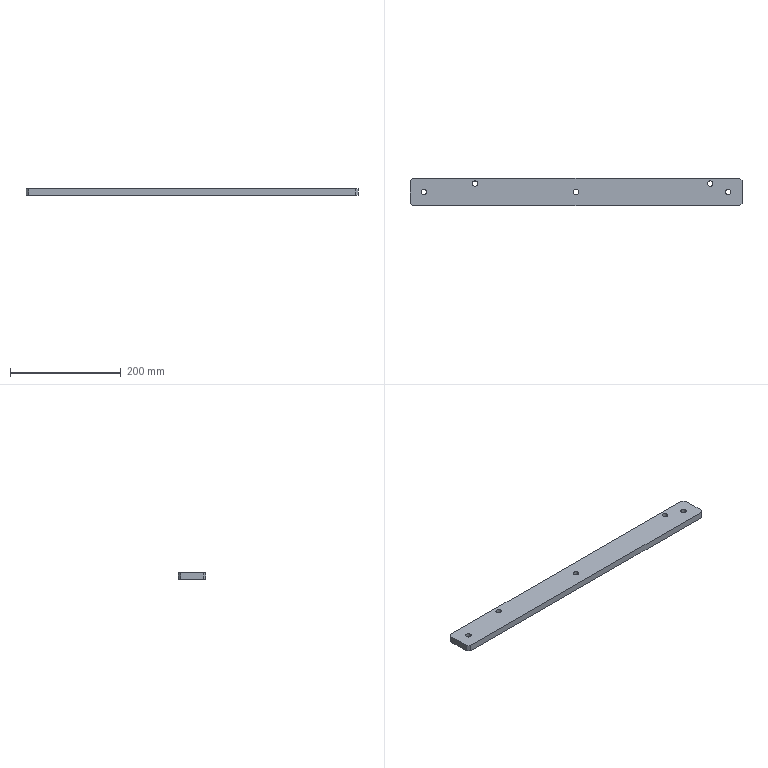Part | STEP file | [01]-6 | 1 solid | 20 faces | box 600 x 50 x 12 mm | volume 354688 mm3 | cylinder 10 | plane 10 | commonest cylinder face diameters 10 x10
STEP:
#1=CARTESIAN_POINT('',(112.5,40.,0.));
#2=VERTEX_POINT('',#1);
#3=CARTESIAN_POINT('',(122.5,40.,0.));
#4=VERTEX_POINT('',#3);
#5=CARTESIAN_POINT('',(117.5,40.,0.));
#6=DIRECTION('',(0.,0.,1.));
#7=DIRECTION('',(1.,0.,0.));
#8=AXIS2_PLACEMENT_3D('',#5,#6,#7);
#9=CIRCLE('',#8,5.);
#10=EDGE_CURVE('',#2,#4,#9,.T.);
#11=ORIENTED_EDGE('',*,*,#10,.F.);
#12=CARTESIAN_POINT('',(112.5,40.,12.));
#13=VERTEX_POINT('',#12);
#14=CARTESIAN_POINT('',(112.5,40.,0.));
#15=DIRECTION('',(0.,0.,1.));
#16=VECTOR('',#15,1000.);
#17=LINE('',#14,#16);
#18=EDGE_CURVE('',#2,#13,#17,.T.);
#19=ORIENTED_EDGE('',*,*,#18,.T.);
#20=CARTESIAN_POINT('',(122.5,40.,12.));
#21=VERTEX_POINT('',#20);
#22=CARTESIAN_POINT('',(117.5,40.,12.));
#23=DIRECTION('',(0.,0.,-1.));
#24=DIRECTION('',(-1.,0.,0.));
#25=AXIS2_PLACEMENT_3D('',#22,#23,#24);
#26=CIRCLE('',#25,5.);
#27=EDGE_CURVE('',#21,#13,#26,.T.);
#28=ORIENTED_EDGE('',*,*,#27,.F.);
#29=CARTESIAN_POINT('',(122.5,40.,0.));
#30=DIRECTION('',(0.,0.,1.));
#31=VECTOR('',#30,1000.);
#32=LINE('',#29,#31);
#33=EDGE_CURVE('',#4,#21,#32,.T.);
#34=ORIENTED_EDGE('',*,*,#33,.F.);
#35=EDGE_LOOP('',(#11,#19,#28,#34));
#36=FACE_OUTER_BOUND('',#35,.T.);
#37=CARTESIAN_POINT('',(117.5,40.,0.));
#38=DIRECTION('',(0.,0.,1.));
#39=DIRECTION('',(1.,0.,0.));
#40=AXIS2_PLACEMENT_3D('',#37,#38,#39);
#41=CYLINDRICAL_SURFACE('',#40,5.);
#42=ADVANCED_FACE('',(#36),#41,.F.);
#43=CARTESIAN_POINT('',(537.5,40.,0.));
#44=VERTEX_POINT('',#43);
#45=CARTESIAN_POINT('',(547.5,40.,0.));
#46=VERTEX_POINT('',#45);
#47=CARTESIAN_POINT('',(542.5,40.,0.));
#48=DIRECTION('',(0.,0.,1.));
#49=DIRECTION('',(1.,0.,0.));
#50=AXIS2_PLACEMENT_3D('',#47,#48,#49);
#51=CIRCLE('',#50,5.);
#52=EDGE_CURVE('',#44,#46,#51,.T.);
#53=ORIENTED_EDGE('',*,*,#52,.F.);
#54=CARTESIAN_POINT('',(537.5,40.,12.));
#55=VERTEX_POINT('',#54);
#56=CARTESIAN_POINT('',(537.5,40.,0.));
#57=DIRECTION('',(0.,0.,1.));
#58=VECTOR('',#57,1000.);
#59=LINE('',#56,#58);
#60=EDGE_CURVE('',#44,#55,#59,.T.);
#61=ORIENTED_EDGE('',*,*,#60,.T.);
#62=CARTESIAN_POINT('',(547.5,40.,12.));
#63=VERTEX_POINT('',#62);
#64=CARTESIAN_POINT('',(542.5,40.,12.));
#65=DIRECTION('',(0.,0.,-1.));
#66=DIRECTION('',(-1.,0.,0.));
#67=AXIS2_PLACEMENT_3D('',#64,#65,#66);
#68=CIRCLE('',#67,5.);
#69=EDGE_CURVE('',#63,#55,#68,.T.);
#70=ORIENTED_EDGE('',*,*,#69,.F.);
#71=CARTESIAN_POINT('',(547.5,40.,0.));
#72=DIRECTION('',(0.,0.,1.));
#73=VECTOR('',#72,1000.);
#74=LINE('',#71,#73);
#75=EDGE_CURVE('',#46,#63,#74,.T.);
#76=ORIENTED_EDGE('',*,*,#75,.F.);
#77=EDGE_LOOP('',(#53,#61,#70,#76));
#78=FACE_OUTER_BOUND('',#77,.T.);
#79=CARTESIAN_POINT('',(542.5,40.,0.));
#80=DIRECTION('',(0.,0.,1.));
#81=DIRECTION('',(1.,0.,0.));
#82=AXIS2_PLACEMENT_3D('',#79,#80,#81);
#83=CYLINDRICAL_SURFACE('',#82,5.);
#84=ADVANCED_FACE('',(#78),#83,.F.);
#85=CARTESIAN_POINT('',(20.,25.,0.));
#86=VERTEX_POINT('',#85);
#87=CARTESIAN_POINT('',(30.,25.,0.));
#88=VERTEX_POINT('',#87);
#89=CARTESIAN_POINT('',(25.,25.,0.));
#90=DIRECTION('',(0.,0.,1.));
#91=DIRECTION('',(1.,0.,0.));
#92=AXIS2_PLACEMENT_3D('',#89,#90,#91);
#93=CIRCLE('',#92,5.);
#94=EDGE_CURVE('',#86,#88,#93,.T.);
#95=ORIENTED_EDGE('',*,*,#94,.F.);
#96=CARTESIAN_POINT('',(20.,25.,12.));
#97=VERTEX_POINT('',#96);
#98=CARTESIAN_POINT('',(20.,25.,0.));
#99=DIRECTION('',(0.,0.,1.));
#100=VECTOR('',#99,1000.);
#101=LINE('',#98,#100);
#102=EDGE_CURVE('',#86,#97,#101,.T.);
#103=ORIENTED_EDGE('',*,*,#102,.T.);
#104=CARTESIAN_POINT('',(30.,25.,12.));
#105=VERTEX_POINT('',#104);
#106=CARTESIAN_POINT('',(25.,25.,12.));
#107=DIRECTION('',(0.,0.,-1.));
#108=DIRECTION('',(-1.,0.,0.));
#109=AXIS2_PLACEMENT_3D('',#106,#107,#108);
#110=CIRCLE('',#109,5.);
#111=EDGE_CURVE('',#105,#97,#110,.T.);
#112=ORIENTED_EDGE('',*,*,#111,.F.);
#113=CARTESIAN_POINT('',(30.,25.,0.));
#114=DIRECTION('',(0.,0.,1.));
#115=VECTOR('',#114,1000.);
#116=LINE('',#113,#115);
#117=EDGE_CURVE('',#88,#105,#116,.T.);
#118=ORIENTED_EDGE('',*,*,#117,.F.);
#119=EDGE_LOOP('',(#95,#103,#112,#118));
#120=FACE_OUTER_BOUND('',#119,.T.);
#121=CARTESIAN_POINT('',(25.,25.,0.));
#122=DIRECTION('',(0.,0.,1.));
#123=DIRECTION('',(1.,0.,0.));
#124=AXIS2_PLACEMENT_3D('',#121,#122,#123);
#125=CYLINDRICAL_SURFACE('',#124,5.);
#126=ADVANCED_FACE('',(#120),#125,.F.);
#127=CARTESIAN_POINT('',(295.,25.,0.));
#128=VERTEX_POINT('',#127);
#129=CARTESIAN_POINT('',(305.,25.,0.));
#130=VERTEX_POINT('',#129);
#131=CARTESIAN_POINT('',(300.,25.,0.));
#132=DIRECTION('',(0.,0.,1.));
#133=DIRECTION('',(1.,0.,0.));
#134=AXIS2_PLACEMENT_3D('',#131,#132,#133);
#135=CIRCLE('',#134,5.);
#136=EDGE_CURVE('',#128,#130,#135,.T.);
#137=ORIENTED_EDGE('',*,*,#136,.F.);
#138=CARTESIAN_POINT('',(295.,25.,12.));
#139=VERTEX_POINT('',#138);
#140=CARTESIAN_POINT('',(295.,25.,0.));
#141=DIRECTION('',(0.,0.,1.));
#142=VECTOR('',#141,1000.);
#143=LINE('',#140,#142);
#144=EDGE_CURVE('',#128,#139,#143,.T.);
#145=ORIENTED_EDGE('',*,*,#144,.T.);
#146=CARTESIAN_POINT('',(305.,25.,12.));
#147=VERTEX_POINT('',#146);
#148=CARTESIAN_POINT('',(300.,25.,12.));
#149=DIRECTION('',(0.,0.,-1.));
#150=DIRECTION('',(-1.,0.,0.));
#151=AXIS2_PLACEMENT_3D('',#148,#149,#150);
#152=CIRCLE('',#151,5.);
#153=EDGE_CURVE('',#147,#139,#152,.T.);
#154=ORIENTED_EDGE('',*,*,#153,.F.);
#155=CARTESIAN_POINT('',(305.,25.,0.));
#156=DIRECTION('',(0.,0.,1.));
#157=VECTOR('',#156,1000.);
#158=LINE('',#155,#157);
#159=EDGE_CURVE('',#130,#147,#158,.T.);
#160=ORIENTED_EDGE('',*,*,#159,.F.);
#161=EDGE_LOOP('',(#137,#145,#154,#160));
#162=FACE_OUTER_BOUND('',#161,.T.);
#163=CARTESIAN_POINT('',(300.,25.,0.));
#164=DIRECTION('',(0.,0.,1.));
#165=DIRECTION('',(1.,0.,0.));
#166=AXIS2_PLACEMENT_3D('',#163,#164,#165);
#167=CYLINDRICAL_SURFACE('',#166,5.);
#168=ADVANCED_FACE('',(#162),#167,.F.);
#169=CARTESIAN_POINT('',(570.,25.,0.));
#170=VERTEX_POINT('',#169);
#171=CARTESIAN_POINT('',(580.,25.,0.));
#172=VERTEX_POINT('',#171);
#173=CARTESIAN_POINT('',(575.,25.,0.));
#174=DIRECTION('',(0.,0.,1.));
#175=DIRECTION('',(1.,0.,0.));
#176=AXIS2_PLACEMENT_3D('',#173,#174,#175);
#177=CIRCLE('',#176,5.);
#178=EDGE_CURVE('',#170,#172,#177,.T.);
#179=ORIENTED_EDGE('',*,*,#178,.F.);
#180=CARTESIAN_POINT('',(570.,25.,12.));
#181=VERTEX_POINT('',#180);
#182=CARTESIAN_POINT('',(570.,25.,0.));
#183=DIRECTION('',(0.,0.,1.));
#184=VECTOR('',#183,1000.);
#185=LINE('',#182,#184);
#186=EDGE_CURVE('',#170,#181,#185,.T.);
#187=ORIENTED_EDGE('',*,*,#186,.T.);
#188=CARTESIAN_POINT('',(580.,25.,12.));
#189=VERTEX_POINT('',#188);
#190=CARTESIAN_POINT('',(575.,25.,12.));
#191=DIRECTION('',(0.,0.,-1.));
#192=DIRECTION('',(-1.,0.,0.));
#193=AXIS2_PLACEMENT_3D('',#190,#191,#192);
#194=CIRCLE('',#193,5.);
#195=EDGE_CURVE('',#189,#181,#194,.T.);
#196=ORIENTED_EDGE('',*,*,#195,.F.);
#197=CARTESIAN_POINT('',(580.,25.,0.));
#198=DIRECTION('',(0.,0.,1.));
#199=VECTOR('',#198,1000.);
#200=LINE('',#197,#199);
#201=EDGE_CURVE('',#172,#189,#200,.T.);
#202=ORIENTED_EDGE('',*,*,#201,.F.);
#203=EDGE_LOOP('',(#179,#187,#196,#202));
#204=FACE_OUTER_BOUND('',#203,.T.);
#205=CARTESIAN_POINT('',(575.,25.,0.));
#206=DIRECTION('',(0.,0.,1.));
#207=DIRECTION('',(1.,0.,0.));
#208=AXIS2_PLACEMENT_3D('',#205,#206,#207);
#209=CYLINDRICAL_SURFACE('',#208,5.);
#210=ADVANCED_FACE('',(#204),#209,.F.);
#211=CARTESIAN_POINT('',(117.5,40.,0.));
#212=DIRECTION('',(0.,0.,1.));
#213=DIRECTION('',(1.,0.,0.));
#214=AXIS2_PLACEMENT_3D('',#211,#212,#213);
#215=CIRCLE('',#214,5.);
#216=EDGE_CURVE('',#4,#2,#215,.T.);
#217=ORIENTED_EDGE('',*,*,#216,.T.);
#218=ORIENTED_EDGE('',*,*,#10,.T.);
#219=EDGE_LOOP('',(#217,#218));
#220=FACE_BOUND('',#219,.T.);
#221=CARTESIAN_POINT('',(542.5,40.,0.));
#222=DIRECTION('',(0.,0.,1.));
#223=DIRECTION('',(1.,0.,0.));
#224=AXIS2_PLACEMENT_3D('',#221,#222,#223);
#225=CIRCLE('',#224,5.);
#226=EDGE_CURVE('',#46,#44,#225,.T.);
#227=ORIENTED_EDGE('',*,*,#226,.T.);
#228=ORIENTED_EDGE('',*,*,#52,.T.);
#229=EDGE_LOOP('',(#227,#228));
#230=FACE_BOUND('',#229,.T.);
#231=CARTESIAN_POINT('',(25.,25.,0.));
#232=DIRECTION('',(0.,0.,1.));
#233=DIRECTION('',(1.,0.,0.));
#234=AXIS2_PLACEMENT_3D('',#231,#232,#233);
#235=CIRCLE('',#234,5.);
#236=EDGE_CURVE('',#88,#86,#235,.T.);
#237=ORIENTED_EDGE('',*,*,#236,.T.);
#238=ORIENTED_EDGE('',*,*,#94,.T.);
#239=EDGE_LOOP('',(#237,#238));
#240=FACE_BOUND('',#239,.T.);
#241=CARTESIAN_POINT('',(300.,25.,0.));
#242=DIRECTION('',(0.,0.,1.));
#243=DIRECTION('',(1.,0.,0.));
#244=AXIS2_PLACEMENT_3D('',#241,#242,#243);
#245=CIRCLE('',#244,5.);
#246=EDGE_CURVE('',#130,#128,#245,.T.);
#247=ORIENTED_EDGE('',*,*,#246,.T.);
#248=ORIENTED_EDGE('',*,*,#136,.T.);
#249=EDGE_LOOP('',(#247,#248));
#250=FACE_BOUND('',#249,.T.);
#251=CARTESIAN_POINT('',(575.,25.,0.));
#252=DIRECTION('',(0.,0.,1.));
#253=DIRECTION('',(1.,0.,0.));
#254=AXIS2_PLACEMENT_3D('',#251,#252,#253);
#255=CIRCLE('',#254,5.);
#256=EDGE_CURVE('',#172,#170,#255,.T.);
#257=ORIENTED_EDGE('',*,*,#256,.T.);
#258=ORIENTED_EDGE('',*,*,#178,.T.);
#259=EDGE_LOOP('',(#257,#258));
#260=FACE_BOUND('',#259,.T.);
#261=CARTESIAN_POINT('',(0.,45.,0.));
#262=VERTEX_POINT('',#261);
#263=CARTESIAN_POINT('',(0.,5.,0.));
#264=VERTEX_POINT('',#263);
#265=CARTESIAN_POINT('',(0.,25.,0.));
#266=DIRECTION('',(0.,-1.,0.));
#267=VECTOR('',#266,1000.);
#268=LINE('',#265,#267);
#269=EDGE_CURVE('',#262,#264,#268,.T.);
#270=ORIENTED_EDGE('',*,*,#269,.F.);
#271=CARTESIAN_POINT('',(5.,50.,0.));
#272=VERTEX_POINT('',#271);
#273=CARTESIAN_POINT('',(140.,185.,0.));
#274=DIRECTION('',(0.7071,0.7071,0.));
#275=VECTOR('',#274,1000.);
#276=LINE('',#273,#275);
#277=EDGE_CURVE('',#262,#272,#276,.T.);
#278=ORIENTED_EDGE('',*,*,#277,.T.);
#279=CARTESIAN_POINT('',(595.,50.,0.));
#280=VERTEX_POINT('',#279);
#281=CARTESIAN_POINT('',(300.,50.,0.));
#282=DIRECTION('',(-1.,0.,0.));
#283=VECTOR('',#282,1000.);
#284=LINE('',#281,#283);
#285=EDGE_CURVE('',#280,#272,#284,.T.);
#286=ORIENTED_EDGE('',*,*,#285,.F.);
#287=CARTESIAN_POINT('',(600.,45.,0.));
#288=VERTEX_POINT('',#287);
#289=CARTESIAN_POINT('',(460.,185.,0.));
#290=DIRECTION('',(0.7071,-0.7071,0.));
#291=VECTOR('',#290,1000.);
#292=LINE('',#289,#291);
#293=EDGE_CURVE('',#280,#288,#292,.T.);
#294=ORIENTED_EDGE('',*,*,#293,.T.);
#295=CARTESIAN_POINT('',(600.,5.,0.));
#296=VERTEX_POINT('',#295);
#297=CARTESIAN_POINT('',(600.,25.,0.));
#298=DIRECTION('',(0.,1.,0.));
#299=VECTOR('',#298,1000.);
#300=LINE('',#297,#299);
#301=EDGE_CURVE('',#296,#288,#300,.T.);
#302=ORIENTED_EDGE('',*,*,#301,.F.);
#303=CARTESIAN_POINT('',(595.,0.,0.));
#304=VERTEX_POINT('',#303);
#305=CARTESIAN_POINT('',(460.,-135.,0.));
#306=DIRECTION('',(-0.7071,-0.7071,0.));
#307=VECTOR('',#306,1000.);
#308=LINE('',#305,#307);
#309=EDGE_CURVE('',#296,#304,#308,.T.);
#310=ORIENTED_EDGE('',*,*,#309,.T.);
#311=CARTESIAN_POINT('',(5.,0.,0.));
#312=VERTEX_POINT('',#311);
#313=CARTESIAN_POINT('',(300.,0.,0.));
#314=DIRECTION('',(1.,0.,0.));
#315=VECTOR('',#314,1000.);
#316=LINE('',#313,#315);
#317=EDGE_CURVE('',#312,#304,#316,.T.);
#318=ORIENTED_EDGE('',*,*,#317,.F.);
#319=CARTESIAN_POINT('',(140.,-135.,0.));
#320=DIRECTION('',(-0.7071,0.7071,0.));
#321=VECTOR('',#320,1000.);
#322=LINE('',#319,#321);
#323=EDGE_CURVE('',#312,#264,#322,.T.);
#324=ORIENTED_EDGE('',*,*,#323,.T.);
#325=EDGE_LOOP('',(#270,#278,#286,#294,#302,#310,#318,#324));
#326=FACE_OUTER_BOUND('',#325,.T.);
#327=CARTESIAN_POINT('',(300.,25.,0.));
#328=DIRECTION('',(0.,0.,-1.));
#329=DIRECTION('',(-1.,0.,0.));
#330=AXIS2_PLACEMENT_3D('',#327,#328,#329);
#331=PLANE('',#330);
#332=ADVANCED_FACE('',(#220,#230,#240,#250,#260,#326),#331,.T.);
#333=ORIENTED_EDGE('',*,*,#317,.T.);
#334=CARTESIAN_POINT('',(595.,0.,12.));
#335=VERTEX_POINT('',#334);
#336=CARTESIAN_POINT('',(595.,0.,12.));
#337=DIRECTION('',(0.,0.,1.));
#338=VECTOR('',#337,1000.);
#339=LINE('',#336,#338);
#340=EDGE_CURVE('',#304,#335,#339,.T.);
#341=ORIENTED_EDGE('',*,*,#340,.T.);
#342=CARTESIAN_POINT('',(5.,0.,12.));
#343=VERTEX_POINT('',#342);
#344=CARTESIAN_POINT('',(300.,0.,12.));
#345=DIRECTION('',(-1.,0.,0.));
#346=VECTOR('',#345,1000.);
#347=LINE('',#344,#346);
#348=EDGE_CURVE('',#335,#343,#347,.T.);
#349=ORIENTED_EDGE('',*,*,#348,.T.);
#350=CARTESIAN_POINT('',(5.,0.,12.));
#351=DIRECTION('',(0.,0.,-1.));
#352=VECTOR('',#351,1000.);
#353=LINE('',#350,#352);
#354=EDGE_CURVE('',#343,#312,#353,.T.);
#355=ORIENTED_EDGE('',*,*,#354,.T.);
#356=EDGE_LOOP('',(#333,#341,#349,#355));
#357=FACE_OUTER_BOUND('',#356,.T.);
#358=CARTESIAN_POINT('',(300.,0.,12.));
#359=DIRECTION('',(0.,-1.,0.));
#360=DIRECTION('',(0.,0.,1.));
#361=AXIS2_PLACEMENT_3D('',#358,#359,#360);
#362=PLANE('',#361);
#363=ADVANCED_FACE('',(#357),#362,.T.);
#364=ORIENTED_EDGE('',*,*,#301,.T.);
#365=CARTESIAN_POINT('',(600.,45.,12.));
#366=VERTEX_POINT('',#365);
#367=CARTESIAN_POINT('',(600.,45.,12.));
#368=DIRECTION('',(0.,0.,1.));
#369=VECTOR('',#368,1000.);
#370=LINE('',#367,#369);
#371=EDGE_CURVE('',#288,#366,#370,.T.);
#372=ORIENTED_EDGE('',*,*,#371,.T.);
#373=CARTESIAN_POINT('',(600.,5.,12.));
#374=VERTEX_POINT('',#373);
#375=CARTESIAN_POINT('',(600.,25.,12.));
#376=DIRECTION('',(0.,-1.,0.));
#377=VECTOR('',#376,1000.);
#378=LINE('',#375,#377);
#379=EDGE_CURVE('',#366,#374,#378,.T.);
#380=ORIENTED_EDGE('',*,*,#379,.T.);
#381=CARTESIAN_POINT('',(600.,5.,12.));
#382=DIRECTION('',(0.,0.,-1.));
#383=VECTOR('',#382,1000.);
#384=LINE('',#381,#383);
#385=EDGE_CURVE('',#374,#296,#384,.T.);
#386=ORIENTED_EDGE('',*,*,#385,.T.);
#387=EDGE_LOOP('',(#364,#372,#380,#386));
#388=FACE_OUTER_BOUND('',#387,.T.);
#389=CARTESIAN_POINT('',(600.,25.,12.));
#390=DIRECTION('',(1.,0.,0.));
#391=DIRECTION('',(0.,0.,-1.));
#392=AXIS2_PLACEMENT_3D('',#389,#390,#391);
#393=PLANE('',#392);
#394=ADVANCED_FACE('',(#388),#393,.T.);
#395=ORIENTED_EDGE('',*,*,#285,.T.);
#396=CARTESIAN_POINT('',(5.,50.,12.));
#397=VERTEX_POINT('',#396);
#398=CARTESIAN_POINT('',(5.,50.,12.));
#399=DIRECTION('',(0.,0.,1.));
#400=VECTOR('',#399,1000.);
#401=LINE('',#398,#400);
#402=EDGE_CURVE('',#272,#397,#401,.T.);
#403=ORIENTED_EDGE('',*,*,#402,.T.);
#404=CARTESIAN_POINT('',(595.,50.,12.));
#405=VERTEX_POINT('',#404);
#406=CARTESIAN_POINT('',(300.,50.,12.));
#407=DIRECTION('',(1.,0.,0.));
#408=VECTOR('',#407,1000.);
#409=LINE('',#406,#408);
#410=EDGE_CURVE('',#397,#405,#409,.T.);
#411=ORIENTED_EDGE('',*,*,#410,.T.);
#412=CARTESIAN_POINT('',(595.,50.,12.));
#413=DIRECTION('',(0.,0.,-1.));
#414=VECTOR('',#413,1000.);
#415=LINE('',#412,#414);
#416=EDGE_CURVE('',#405,#280,#415,.T.);
#417=ORIENTED_EDGE('',*,*,#416,.T.);
#418=EDGE_LOOP('',(#395,#403,#411,#417));
#419=FACE_OUTER_BOUND('',#418,.T.);
#420=CARTESIAN_POINT('',(300.,50.,12.));
#421=DIRECTION('',(0.,1.,0.));
#422=DIRECTION('',(0.,0.,-1.));
#423=AXIS2_PLACEMENT_3D('',#420,#421,#422);
#424=PLANE('',#423);
#425=ADVANCED_FACE('',(#419),#424,.T.);
#426=ORIENTED_EDGE('',*,*,#27,.T.);
#427=CARTESIAN_POINT('',(117.5,40.,12.));
#428=DIRECTION('',(0.,0.,-1.));
#429=DIRECTION('',(-1.,0.,0.));
#430=AXIS2_PLACEMENT_3D('',#427,#428,#429);
#431=CIRCLE('',#430,5.);
#432=EDGE_CURVE('',#13,#21,#431,.T.);
#433=ORIENTED_EDGE('',*,*,#432,.T.);
#434=EDGE_LOOP('',(#426,#433));
#435=FACE_BOUND('',#434,.T.);
#436=ORIENTED_EDGE('',*,*,#69,.T.);
#437=CARTESIAN_POINT('',(542.5,40.,12.));
#438=DIRECTION('',(0.,0.,-1.));
#439=DIRECTION('',(-1.,0.,0.));
#440=AXIS2_PLACEMENT_3D('',#437,#438,#439);
#441=CIRCLE('',#440,5.);
#442=EDGE_CURVE('',#55,#63,#441,.T.);
#443=ORIENTED_EDGE('',*,*,#442,.T.);
#444=EDGE_LOOP('',(#436,#443));
#445=FACE_BOUND('',#444,.T.);
#446=ORIENTED_EDGE('',*,*,#111,.T.);
#447=CARTESIAN_POINT('',(25.,25.,12.));
#448=DIRECTION('',(0.,0.,-1.));
#449=DIRECTION('',(-1.,0.,0.));
#450=AXIS2_PLACEMENT_3D('',#447,#448,#449);
#451=CIRCLE('',#450,5.);
#452=EDGE_CURVE('',#97,#105,#451,.T.);
#453=ORIENTED_EDGE('',*,*,#452,.T.);
#454=EDGE_LOOP('',(#446,#453));
#455=FACE_BOUND('',#454,.T.);
#456=ORIENTED_EDGE('',*,*,#153,.T.);
#457=CARTESIAN_POINT('',(300.,25.,12.));
#458=DIRECTION('',(0.,0.,-1.));
#459=DIRECTION('',(-1.,0.,0.));
#460=AXIS2_PLACEMENT_3D('',#457,#458,#459);
#461=CIRCLE('',#460,5.);
#462=EDGE_CURVE('',#139,#147,#461,.T.);
#463=ORIENTED_EDGE('',*,*,#462,.T.);
#464=EDGE_LOOP('',(#456,#463));
#465=FACE_BOUND('',#464,.T.);
#466=ORIENTED_EDGE('',*,*,#195,.T.);
#467=CARTESIAN_POINT('',(575.,25.,12.));
#468=DIRECTION('',(0.,0.,-1.));
#469=DIRECTION('',(-1.,0.,0.));
#470=AXIS2_PLACEMENT_3D('',#467,#468,#469);
#471=CIRCLE('',#470,5.);
#472=EDGE_CURVE('',#181,#189,#471,.T.);
#473=ORIENTED_EDGE('',*,*,#472,.T.);
#474=EDGE_LOOP('',(#466,#473));
#475=FACE_BOUND('',#474,.T.);
#476=ORIENTED_EDGE('',*,*,#410,.F.);
#477=CARTESIAN_POINT('',(0.,45.,12.));
#478=VERTEX_POINT('',#477);
#479=CARTESIAN_POINT('',(140.,185.,12.));
#480=DIRECTION('',(-0.7071,-0.7071,0.));
#481=VECTOR('',#480,1000.);
#482=LINE('',#479,#481);
#483=EDGE_CURVE('',#397,#478,#482,.T.);
#484=ORIENTED_EDGE('',*,*,#483,.T.);
#485=CARTESIAN_POINT('',(0.,5.,12.));
#486=VERTEX_POINT('',#485);
#487=CARTESIAN_POINT('',(0.,25.,12.));
#488=DIRECTION('',(0.,1.,0.));
#489=VECTOR('',#488,1000.);
#490=LINE('',#487,#489);
#491=EDGE_CURVE('',#486,#478,#490,.T.);
#492=ORIENTED_EDGE('',*,*,#491,.F.);
#493=CARTESIAN_POINT('',(140.,-135.,12.));
#494=DIRECTION('',(0.7071,-0.7071,0.));
#495=VECTOR('',#494,1000.);
#496=LINE('',#493,#495);
#497=EDGE_CURVE('',#486,#343,#496,.T.);
#498=ORIENTED_EDGE('',*,*,#497,.T.);
#499=ORIENTED_EDGE('',*,*,#348,.F.);
#500=CARTESIAN_POINT('',(460.,-135.,12.));
#501=DIRECTION('',(0.7071,0.7071,0.));
#502=VECTOR('',#501,1000.);
#503=LINE('',#500,#502);
#504=EDGE_CURVE('',#335,#374,#503,.T.);
#505=ORIENTED_EDGE('',*,*,#504,.T.);
#506=ORIENTED_EDGE('',*,*,#379,.F.);
#507=CARTESIAN_POINT('',(460.,185.,12.));
#508=DIRECTION('',(-0.7071,0.7071,0.));
#509=VECTOR('',#508,1000.);
#510=LINE('',#507,#509);
#511=EDGE_CURVE('',#366,#405,#510,.T.);
#512=ORIENTED_EDGE('',*,*,#511,.T.);
#513=EDGE_LOOP('',(#476,#484,#492,#498,#499,#505,#506,#512));
#514=FACE_OUTER_BOUND('',#513,.T.);
#515=CARTESIAN_POINT('',(300.,25.,12.));
#516=DIRECTION('',(0.,0.,1.));
#517=DIRECTION('',(1.,0.,0.));
#518=AXIS2_PLACEMENT_3D('',#515,#516,#517);
#519=PLANE('',#518);
#520=ADVANCED_FACE('',(#435,#445,#455,#465,#475,#514),#519,.T.);
#521=ORIENTED_EDGE('',*,*,#491,.T.);
#522=CARTESIAN_POINT('',(0.,45.,12.));
#523=DIRECTION('',(0.,0.,-1.));
#524=VECTOR('',#523,1000.);
#525=LINE('',#522,#524);
#526=EDGE_CURVE('',#478,#262,#525,.T.);
#527=ORIENTED_EDGE('',*,*,#526,.T.);
#528=ORIENTED_EDGE('',*,*,#269,.T.);
#529=CARTESIAN_POINT('',(0.,5.,12.));
#530=DIRECTION('',(0.,0.,1.));
#531=VECTOR('',#530,1000.);
#532=LINE('',#529,#531);
#533=EDGE_CURVE('',#264,#486,#532,.T.);
#534=ORIENTED_EDGE('',*,*,#533,.T.);
#535=EDGE_LOOP('',(#521,#527,#528,#534));
#536=FACE_OUTER_BOUND('',#535,.T.);
#537=CARTESIAN_POINT('',(0.,25.,12.));
#538=DIRECTION('',(-1.,0.,0.));
#539=DIRECTION('',(0.,0.,1.));
#540=AXIS2_PLACEMENT_3D('',#537,#538,#539);
#541=PLANE('',#540);
#542=ADVANCED_FACE('',(#536),#541,.T.);
#543=ORIENTED_EDGE('',*,*,#497,.F.);
#544=ORIENTED_EDGE('',*,*,#533,.F.);
#545=ORIENTED_EDGE('',*,*,#323,.F.);
#546=ORIENTED_EDGE('',*,*,#354,.F.);
#547=EDGE_LOOP('',(#543,#544,#545,#546));
#548=FACE_OUTER_BOUND('',#547,.T.);
#549=CARTESIAN_POINT('',(5.,0.,12.));
#550=DIRECTION('',(0.7071,0.7071,0.));
#551=DIRECTION('',(0.,0.,-1.));
#552=AXIS2_PLACEMENT_3D('',#549,#550,#551);
#553=PLANE('',#552);
#554=ADVANCED_FACE('',(#548),#553,.F.);
#555=ORIENTED_EDGE('',*,*,#504,.F.);
#556=ORIENTED_EDGE('',*,*,#340,.F.);
#557=ORIENTED_EDGE('',*,*,#309,.F.);
#558=ORIENTED_EDGE('',*,*,#385,.F.);
#559=EDGE_LOOP('',(#555,#556,#557,#558));
#560=FACE_OUTER_BOUND('',#559,.T.);
#561=CARTESIAN_POINT('',(600.,5.,12.));
#562=DIRECTION('',(-0.7071,0.7071,0.));
#563=DIRECTION('',(0.,0.,-1.));
#564=AXIS2_PLACEMENT_3D('',#561,#562,#563);
#565=PLANE('',#564);
#566=ADVANCED_FACE('',(#560),#565,.F.);
#567=ORIENTED_EDGE('',*,*,#511,.F.);
#568=ORIENTED_EDGE('',*,*,#371,.F.);
#569=ORIENTED_EDGE('',*,*,#293,.F.);
#570=ORIENTED_EDGE('',*,*,#416,.F.);
#571=EDGE_LOOP('',(#567,#568,#569,#570));
#572=FACE_OUTER_BOUND('',#571,.T.);
#573=CARTESIAN_POINT('',(595.,50.,12.));
#574=DIRECTION('',(-0.7071,-0.7071,0.));
#575=DIRECTION('',(0.,0.,-1.));
#576=AXIS2_PLACEMENT_3D('',#573,#574,#575);
#577=PLANE('',#576);
#578=ADVANCED_FACE('',(#572),#577,.F.);
#579=ORIENTED_EDGE('',*,*,#483,.F.);
#580=ORIENTED_EDGE('',*,*,#402,.F.);
#581=ORIENTED_EDGE('',*,*,#277,.F.);
#582=ORIENTED_EDGE('',*,*,#526,.F.);
#583=EDGE_LOOP('',(#579,#580,#581,#582));
#584=FACE_OUTER_BOUND('',#583,.T.);
#585=CARTESIAN_POINT('',(0.,45.,12.));
#586=DIRECTION('',(0.7071,-0.7071,0.));
#587=DIRECTION('',(0.,0.,-1.));
#588=AXIS2_PLACEMENT_3D('',#585,#586,#587);
#589=PLANE('',#588);
#590=ADVANCED_FACE('',(#584),#589,.F.);
#591=ORIENTED_EDGE('',*,*,#186,.F.);
#592=ORIENTED_EDGE('',*,*,#256,.F.);
#593=ORIENTED_EDGE('',*,*,#201,.T.);
#594=ORIENTED_EDGE('',*,*,#472,.F.);
#595=EDGE_LOOP('',(#591,#592,#593,#594));
#596=FACE_OUTER_BOUND('',#595,.T.);
#597=CARTESIAN_POINT('',(575.,25.,0.));
#598=DIRECTION('',(0.,0.,1.));
#599=DIRECTION('',(1.,0.,0.));
#600=AXIS2_PLACEMENT_3D('',#597,#598,#599);
#601=CYLINDRICAL_SURFACE('',#600,5.);
#602=ADVANCED_FACE('',(#596),#601,.F.);
#603=ORIENTED_EDGE('',*,*,#144,.F.);
#604=ORIENTED_EDGE('',*,*,#246,.F.);
#605=ORIENTED_EDGE('',*,*,#159,.T.);
#606=ORIENTED_EDGE('',*,*,#462,.F.);
#607=EDGE_LOOP('',(#603,#604,#605,#606));
#608=FACE_OUTER_BOUND('',#607,.T.);
#609=CARTESIAN_POINT('',(300.,25.,0.));
#610=DIRECTION('',(0.,0.,1.));
#611=DIRECTION('',(1.,0.,0.));
#612=AXIS2_PLACEMENT_3D('',#609,#610,#611);
#613=CYLINDRICAL_SURFACE('',#612,5.);
#614=ADVANCED_FACE('',(#608),#613,.F.);
#615=ORIENTED_EDGE('',*,*,#102,.F.);
#616=ORIENTED_EDGE('',*,*,#236,.F.);
#617=ORIENTED_EDGE('',*,*,#117,.T.);
#618=ORIENTED_EDGE('',*,*,#452,.F.);
#619=EDGE_LOOP('',(#615,#616,#617,#618));
#620=FACE_OUTER_BOUND('',#619,.T.);
#621=CARTESIAN_POINT('',(25.,25.,0.));
#622=DIRECTION('',(0.,0.,1.));
#623=DIRECTION('',(1.,0.,0.));
#624=AXIS2_PLACEMENT_3D('',#621,#622,#623);
#625=CYLINDRICAL_SURFACE('',#624,5.);
#626=ADVANCED_FACE('',(#620),#625,.F.);
#627=ORIENTED_EDGE('',*,*,#60,.F.);
#628=ORIENTED_EDGE('',*,*,#226,.F.);
#629=ORIENTED_EDGE('',*,*,#75,.T.);
#630=ORIENTED_EDGE('',*,*,#442,.F.);
#631=EDGE_LOOP('',(#627,#628,#629,#630));
#632=FACE_OUTER_BOUND('',#631,.T.);
#633=CARTESIAN_POINT('',(542.5,40.,0.));
#634=DIRECTION('',(0.,0.,1.));
#635=DIRECTION('',(1.,0.,0.));
#636=AXIS2_PLACEMENT_3D('',#633,#634,#635);
#637=CYLINDRICAL_SURFACE('',#636,5.);
#638=ADVANCED_FACE('',(#632),#637,.F.);
#639=ORIENTED_EDGE('',*,*,#18,.F.);
#640=ORIENTED_EDGE('',*,*,#216,.F.);
#641=ORIENTED_EDGE('',*,*,#33,.T.);
#642=ORIENTED_EDGE('',*,*,#432,.F.);
#643=EDGE_LOOP('',(#639,#640,#641,#642));
#644=FACE_OUTER_BOUND('',#643,.T.);
#645=CARTESIAN_POINT('',(117.5,40.,0.));
#646=DIRECTION('',(0.,0.,1.));
#647=DIRECTION('',(1.,0.,0.));
#648=AXIS2_PLACEMENT_3D('',#645,#646,#647);
#649=CYLINDRICAL_SURFACE('',#648,5.);
#650=ADVANCED_FACE('',(#644),#649,.F.);
#651=CLOSED_SHELL('',(#42,#84,#126,#168,#210,#332,#363,#394,#425,#520,#542,#554,#566,#578,#590,#602,#614,#626,#638,#650));
#652=MANIFOLD_SOLID_BREP('',#651);
#653=CARTESIAN_POINT('',(0.,0.,0.));
#654=DIRECTION('',(0.,0.,1.));
#655=DIRECTION('',(1.,0.,0.));
#656=AXIS2_PLACEMENT_3D('',#653,#654,#655);
#657=(LENGTH_UNIT()NAMED_UNIT(*)SI_UNIT(.MILLI.,.METRE.));
#658=UNCERTAINTY_MEASURE_WITH_UNIT(LENGTH_MEASURE(0.00001),#657,'','');
#659=(NAMED_UNIT(*)PLANE_ANGLE_UNIT()SI_UNIT($,.RADIAN.));
#660=(NAMED_UNIT(*)SI_UNIT($,.STERADIAN.)SOLID_ANGLE_UNIT());
#661=(GEOMETRIC_REPRESENTATION_CONTEXT(3)GLOBAL_UNCERTAINTY_ASSIGNED_CONTEXT((#658))GLOBAL_UNIT_ASSIGNED_CONTEXT((#657,#659,#660))REPRESENTATION_CONTEXT('',''));
#662=ADVANCED_BREP_SHAPE_REPRESENTATION('',(#652,#656),#661);